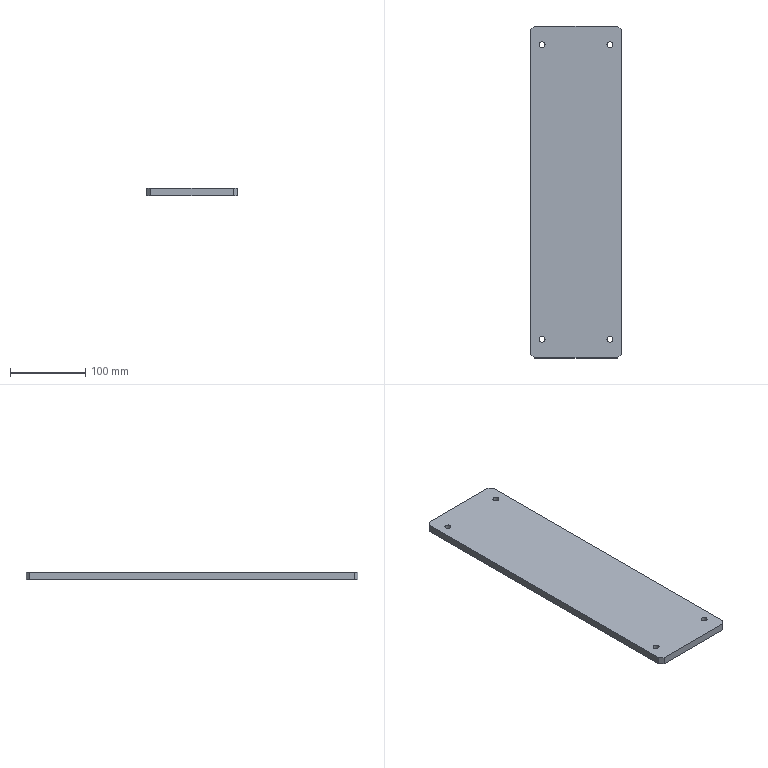Part | STEP file | POST.PLATE.2.stp | 1 solid | 18 faces | box 120 x 440 x 10 mm | volume 525489 mm3 | spline 10 | cylinder 4 | plane 4 | commonest cylinder face diameters 8 x4